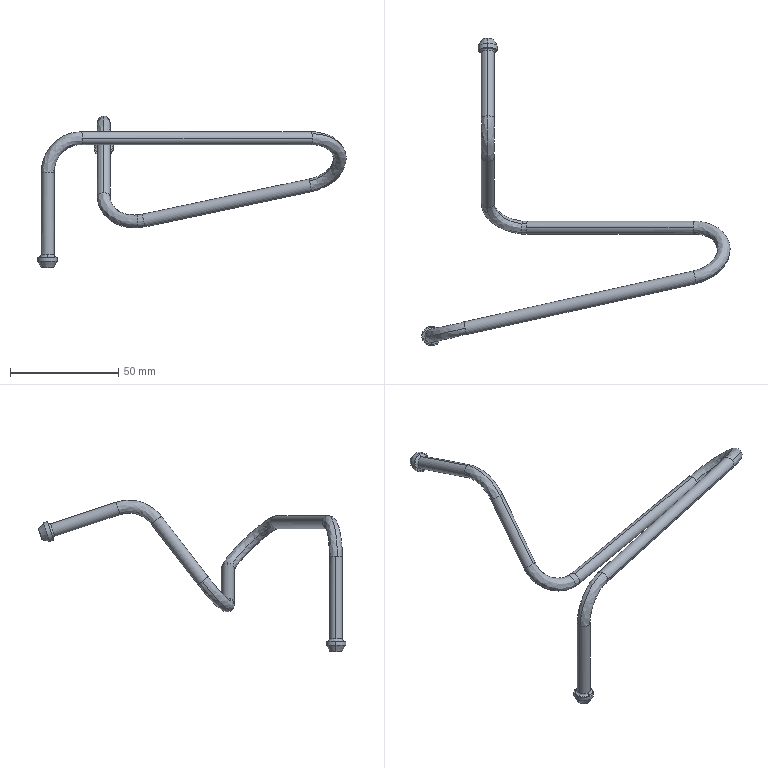Part | SolidWorks | features BaseBody 1 | 1 solid | 64 faces | box 142.709 x 142.113 x 70.221 mm | volume 11431 mm3 | cylinder 28 | spline 24 | cone 8 | plane 4 | commonest cylinder face diameters 1.5 x10 6 x10 2 x4 9 x4